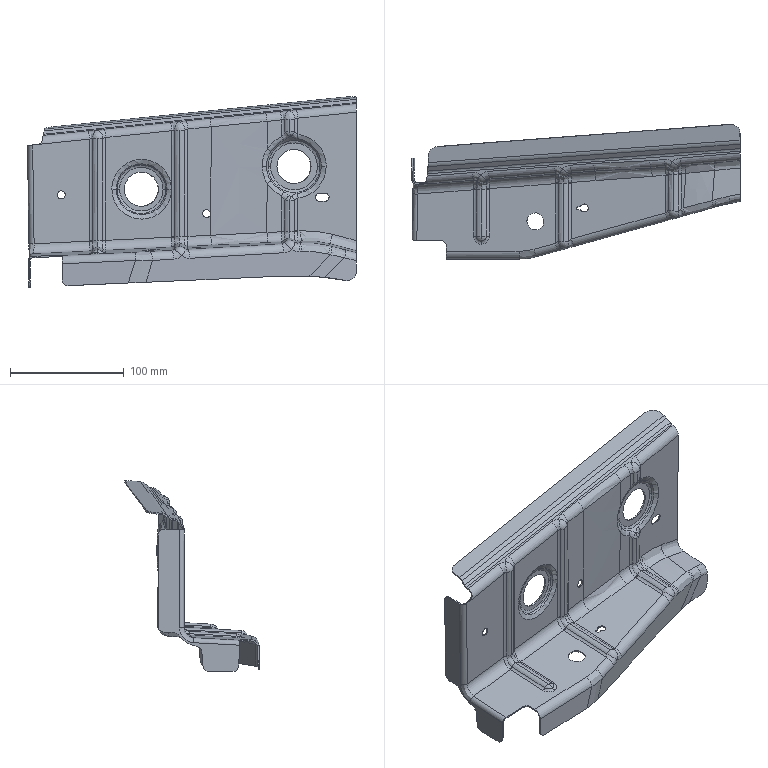Part | 1 solid | 367 faces | box 288.755 x 118.551 x 167.538 mm | volume 76920 mm3 | spline 228 | cylinder 83 | plane 41 | other 7 | sphere 4 | torus 4 | commonest cylinder face diameters 7.6 x14 10 x14 12 x11 14.4 x10 7 x5 17.6 x5